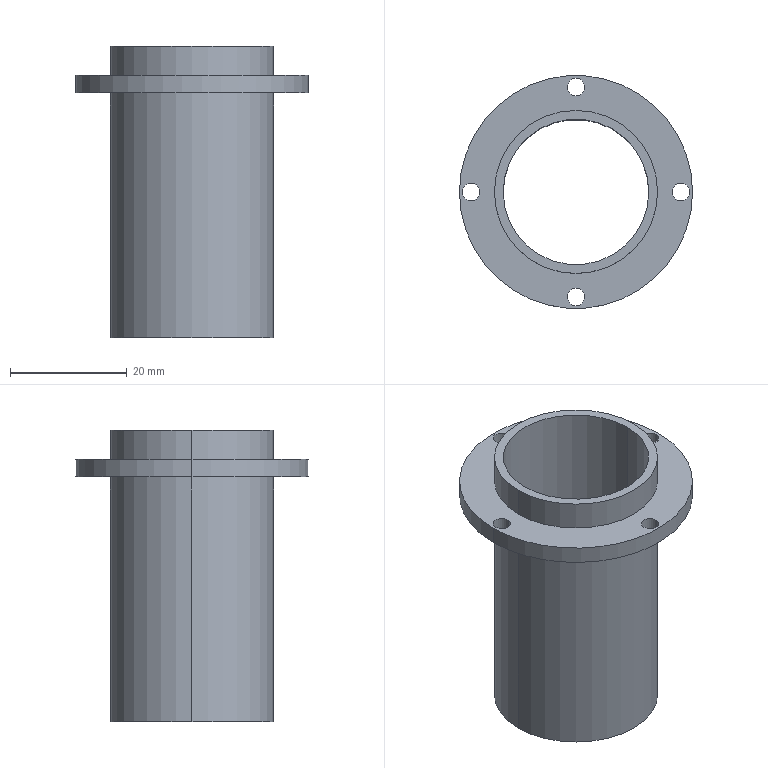Part | SolidWorks | features Extrusion 1, ICE 1 | 1 solid | 20 faces | box 40 x 40 x 50 mm | volume 8082 mm3 | cylinder 16 | plane 4 | commonest cylinder face diameters 3 x8 28 x4 25 x2 40 x2
STEP:
#1=CARTESIAN_POINT('',(-19.5,0.,17.));
#2=VERTEX_POINT('',#1);
#3=CARTESIAN_POINT('',(-16.5,0.,17.));
#4=VERTEX_POINT('',#3);
#5=CARTESIAN_POINT('',(-18.,0.,17.));
#6=DIRECTION('',(0.,0.,1.));
#7=DIRECTION('',(1.,0.,0.));
#8=AXIS2_PLACEMENT_3D('',#5,#6,#7);
#9=CIRCLE('',#8,1.5);
#10=EDGE_CURVE('',#2,#4,#9,.T.);
#11=ORIENTED_EDGE('',*,*,#10,.F.);
#12=CARTESIAN_POINT('',(-19.5,0.,20.));
#13=VERTEX_POINT('',#12);
#14=CARTESIAN_POINT('',(-19.5,0.,17.));
#15=DIRECTION('',(0.,0.,1.));
#16=VECTOR('',#15,1000.);
#17=LINE('',#14,#16);
#18=EDGE_CURVE('',#2,#13,#17,.T.);
#19=ORIENTED_EDGE('',*,*,#18,.T.);
#20=CARTESIAN_POINT('',(-16.5,0.,20.));
#21=VERTEX_POINT('',#20);
#22=CARTESIAN_POINT('',(-18.,0.,20.));
#23=DIRECTION('',(0.,0.,1.));
#24=DIRECTION('',(1.,0.,0.));
#25=AXIS2_PLACEMENT_3D('',#22,#23,#24);
#26=CIRCLE('',#25,1.5);
#27=EDGE_CURVE('',#13,#21,#26,.T.);
#28=ORIENTED_EDGE('',*,*,#27,.T.);
#29=CARTESIAN_POINT('',(-16.5,0.,17.));
#30=DIRECTION('',(0.,0.,1.));
#31=VECTOR('',#30,1000.);
#32=LINE('',#29,#31);
#33=EDGE_CURVE('',#4,#21,#32,.T.);
#34=ORIENTED_EDGE('',*,*,#33,.F.);
#35=EDGE_LOOP('',(#11,#19,#28,#34));
#36=FACE_OUTER_BOUND('',#35,.T.);
#37=CARTESIAN_POINT('',(-18.,0.,17.));
#38=DIRECTION('',(0.,0.,1.));
#39=DIRECTION('',(1.,0.,0.));
#40=AXIS2_PLACEMENT_3D('',#37,#38,#39);
#41=CYLINDRICAL_SURFACE('',#40,1.5);
#42=ADVANCED_FACE('',(#36),#41,.F.);
#43=CARTESIAN_POINT('',(-1.5,-18.,17.));
#44=VERTEX_POINT('',#43);
#45=CARTESIAN_POINT('',(1.5,-18.,17.));
#46=VERTEX_POINT('',#45);
#47=CARTESIAN_POINT('',(0.,-18.,17.));
#48=DIRECTION('',(0.,0.,1.));
#49=DIRECTION('',(1.,0.,0.));
#50=AXIS2_PLACEMENT_3D('',#47,#48,#49);
#51=CIRCLE('',#50,1.5);
#52=EDGE_CURVE('',#44,#46,#51,.T.);
#53=ORIENTED_EDGE('',*,*,#52,.F.);
#54=CARTESIAN_POINT('',(-1.5,-18.,20.));
#55=VERTEX_POINT('',#54);
#56=CARTESIAN_POINT('',(-1.5,-18.,17.));
#57=DIRECTION('',(0.,0.,1.));
#58=VECTOR('',#57,1000.);
#59=LINE('',#56,#58);
#60=EDGE_CURVE('',#44,#55,#59,.T.);
#61=ORIENTED_EDGE('',*,*,#60,.T.);
#62=CARTESIAN_POINT('',(1.5,-18.,20.));
#63=VERTEX_POINT('',#62);
#64=CARTESIAN_POINT('',(0.,-18.,20.));
#65=DIRECTION('',(0.,0.,1.));
#66=DIRECTION('',(1.,0.,0.));
#67=AXIS2_PLACEMENT_3D('',#64,#65,#66);
#68=CIRCLE('',#67,1.5);
#69=EDGE_CURVE('',#55,#63,#68,.T.);
#70=ORIENTED_EDGE('',*,*,#69,.T.);
#71=CARTESIAN_POINT('',(1.5,-18.,17.));
#72=DIRECTION('',(0.,0.,1.));
#73=VECTOR('',#72,1000.);
#74=LINE('',#71,#73);
#75=EDGE_CURVE('',#46,#63,#74,.T.);
#76=ORIENTED_EDGE('',*,*,#75,.F.);
#77=EDGE_LOOP('',(#53,#61,#70,#76));
#78=FACE_OUTER_BOUND('',#77,.T.);
#79=CARTESIAN_POINT('',(0.,-18.,17.));
#80=DIRECTION('',(0.,0.,1.));
#81=DIRECTION('',(1.,0.,0.));
#82=AXIS2_PLACEMENT_3D('',#79,#80,#81);
#83=CYLINDRICAL_SURFACE('',#82,1.5);
#84=ADVANCED_FACE('',(#78),#83,.F.);
#85=CARTESIAN_POINT('',(16.5,0.,17.));
#86=VERTEX_POINT('',#85);
#87=CARTESIAN_POINT('',(19.5,0.,17.));
#88=VERTEX_POINT('',#87);
#89=CARTESIAN_POINT('',(18.,0.,17.));
#90=DIRECTION('',(0.,0.,1.));
#91=DIRECTION('',(1.,0.,0.));
#92=AXIS2_PLACEMENT_3D('',#89,#90,#91);
#93=CIRCLE('',#92,1.5);
#94=EDGE_CURVE('',#86,#88,#93,.T.);
#95=ORIENTED_EDGE('',*,*,#94,.F.);
#96=CARTESIAN_POINT('',(16.5,0.,20.));
#97=VERTEX_POINT('',#96);
#98=CARTESIAN_POINT('',(16.5,0.,17.));
#99=DIRECTION('',(0.,0.,1.));
#100=VECTOR('',#99,1000.);
#101=LINE('',#98,#100);
#102=EDGE_CURVE('',#86,#97,#101,.T.);
#103=ORIENTED_EDGE('',*,*,#102,.T.);
#104=CARTESIAN_POINT('',(19.5,0.,20.));
#105=VERTEX_POINT('',#104);
#106=CARTESIAN_POINT('',(18.,0.,20.));
#107=DIRECTION('',(0.,0.,1.));
#108=DIRECTION('',(1.,0.,0.));
#109=AXIS2_PLACEMENT_3D('',#106,#107,#108);
#110=CIRCLE('',#109,1.5);
#111=EDGE_CURVE('',#97,#105,#110,.T.);
#112=ORIENTED_EDGE('',*,*,#111,.T.);
#113=CARTESIAN_POINT('',(19.5,0.,17.));
#114=DIRECTION('',(0.,0.,1.));
#115=VECTOR('',#114,1000.);
#116=LINE('',#113,#115);
#117=EDGE_CURVE('',#88,#105,#116,.T.);
#118=ORIENTED_EDGE('',*,*,#117,.F.);
#119=EDGE_LOOP('',(#95,#103,#112,#118));
#120=FACE_OUTER_BOUND('',#119,.T.);
#121=CARTESIAN_POINT('',(18.,0.,17.));
#122=DIRECTION('',(0.,0.,1.));
#123=DIRECTION('',(1.,0.,0.));
#124=AXIS2_PLACEMENT_3D('',#121,#122,#123);
#125=CYLINDRICAL_SURFACE('',#124,1.5);
#126=ADVANCED_FACE('',(#120),#125,.F.);
#127=CARTESIAN_POINT('',(-1.5,18.,17.));
#128=VERTEX_POINT('',#127);
#129=CARTESIAN_POINT('',(1.5,18.,17.));
#130=VERTEX_POINT('',#129);
#131=CARTESIAN_POINT('',(0.,18.,17.));
#132=DIRECTION('',(0.,0.,1.));
#133=DIRECTION('',(1.,0.,0.));
#134=AXIS2_PLACEMENT_3D('',#131,#132,#133);
#135=CIRCLE('',#134,1.5);
#136=EDGE_CURVE('',#128,#130,#135,.T.);
#137=ORIENTED_EDGE('',*,*,#136,.F.);
#138=CARTESIAN_POINT('',(-1.5,18.,20.));
#139=VERTEX_POINT('',#138);
#140=CARTESIAN_POINT('',(-1.5,18.,17.));
#141=DIRECTION('',(0.,0.,1.));
#142=VECTOR('',#141,1000.);
#143=LINE('',#140,#142);
#144=EDGE_CURVE('',#128,#139,#143,.T.);
#145=ORIENTED_EDGE('',*,*,#144,.T.);
#146=CARTESIAN_POINT('',(1.5,18.,20.));
#147=VERTEX_POINT('',#146);
#148=CARTESIAN_POINT('',(0.,18.,20.));
#149=DIRECTION('',(0.,0.,1.));
#150=DIRECTION('',(1.,0.,0.));
#151=AXIS2_PLACEMENT_3D('',#148,#149,#150);
#152=CIRCLE('',#151,1.5);
#153=EDGE_CURVE('',#139,#147,#152,.T.);
#154=ORIENTED_EDGE('',*,*,#153,.T.);
#155=CARTESIAN_POINT('',(1.5,18.,17.));
#156=DIRECTION('',(0.,0.,1.));
#157=VECTOR('',#156,1000.);
#158=LINE('',#155,#157);
#159=EDGE_CURVE('',#130,#147,#158,.T.);
#160=ORIENTED_EDGE('',*,*,#159,.F.);
#161=EDGE_LOOP('',(#137,#145,#154,#160));
#162=FACE_OUTER_BOUND('',#161,.T.);
#163=CARTESIAN_POINT('',(0.,18.,17.));
#164=DIRECTION('',(0.,0.,1.));
#165=DIRECTION('',(1.,0.,0.));
#166=AXIS2_PLACEMENT_3D('',#163,#164,#165);
#167=CYLINDRICAL_SURFACE('',#166,1.5);
#168=ADVANCED_FACE('',(#162),#167,.F.);
#169=CARTESIAN_POINT('',(20.,0.,17.));
#170=VERTEX_POINT('',#169);
#171=CARTESIAN_POINT('',(-20.,0.,17.));
#172=VERTEX_POINT('',#171);
#173=CARTESIAN_POINT('',(0.,0.,17.));
#174=DIRECTION('',(0.,0.,1.));
#175=DIRECTION('',(1.,0.,0.));
#176=AXIS2_PLACEMENT_3D('',#173,#174,#175);
#177=CIRCLE('',#176,20.);
#178=EDGE_CURVE('',#170,#172,#177,.T.);
#179=ORIENTED_EDGE('',*,*,#178,.T.);
#180=CARTESIAN_POINT('',(-20.,0.,20.));
#181=VERTEX_POINT('',#180);
#182=CARTESIAN_POINT('',(-20.,0.,17.));
#183=DIRECTION('',(0.,0.,1.));
#184=VECTOR('',#183,1000.);
#185=LINE('',#182,#184);
#186=EDGE_CURVE('',#172,#181,#185,.T.);
#187=ORIENTED_EDGE('',*,*,#186,.T.);
#188=CARTESIAN_POINT('',(20.,0.,20.));
#189=VERTEX_POINT('',#188);
#190=CARTESIAN_POINT('',(0.,0.,20.));
#191=DIRECTION('',(0.,0.,1.));
#192=DIRECTION('',(1.,0.,0.));
#193=AXIS2_PLACEMENT_3D('',#190,#191,#192);
#194=CIRCLE('',#193,20.);
#195=EDGE_CURVE('',#189,#181,#194,.T.);
#196=ORIENTED_EDGE('',*,*,#195,.F.);
#197=CARTESIAN_POINT('',(20.,0.,17.));
#198=DIRECTION('',(0.,0.,1.));
#199=VECTOR('',#198,1000.);
#200=LINE('',#197,#199);
#201=EDGE_CURVE('',#170,#189,#200,.T.);
#202=ORIENTED_EDGE('',*,*,#201,.F.);
#203=EDGE_LOOP('',(#179,#187,#196,#202));
#204=FACE_OUTER_BOUND('',#203,.T.);
#205=CARTESIAN_POINT('',(0.,0.,17.));
#206=DIRECTION('',(0.,0.,1.));
#207=DIRECTION('',(1.,0.,0.));
#208=AXIS2_PLACEMENT_3D('',#205,#206,#207);
#209=CYLINDRICAL_SURFACE('',#208,20.);
#210=ADVANCED_FACE('',(#204),#209,.T.);
#211=CARTESIAN_POINT('',(-12.5,0.,25.));
#212=VERTEX_POINT('',#211);
#213=CARTESIAN_POINT('',(12.5,0.,25.));
#214=VERTEX_POINT('',#213);
#215=CARTESIAN_POINT('',(0.,0.,25.));
#216=DIRECTION('',(0.,0.,1.));
#217=DIRECTION('',(1.,0.,0.));
#218=AXIS2_PLACEMENT_3D('',#215,#216,#217);
#219=CIRCLE('',#218,12.5);
#220=EDGE_CURVE('',#212,#214,#219,.T.);
#221=ORIENTED_EDGE('',*,*,#220,.T.);
#222=CARTESIAN_POINT('',(12.5,0.,-25.));
#223=VERTEX_POINT('',#222);
#224=CARTESIAN_POINT('',(12.5,0.,25.));
#225=DIRECTION('',(0.,0.,-1.));
#226=VECTOR('',#225,1000.);
#227=LINE('',#224,#226);
#228=EDGE_CURVE('',#214,#223,#227,.T.);
#229=ORIENTED_EDGE('',*,*,#228,.T.);
#230=CARTESIAN_POINT('',(-12.5,0.,-25.));
#231=VERTEX_POINT('',#230);
#232=CARTESIAN_POINT('',(0.,0.,-25.));
#233=DIRECTION('',(0.,0.,1.));
#234=DIRECTION('',(1.,0.,0.));
#235=AXIS2_PLACEMENT_3D('',#232,#233,#234);
#236=CIRCLE('',#235,12.5);
#237=EDGE_CURVE('',#231,#223,#236,.T.);
#238=ORIENTED_EDGE('',*,*,#237,.F.);
#239=CARTESIAN_POINT('',(-12.5,0.,25.));
#240=DIRECTION('',(0.,0.,-1.));
#241=VECTOR('',#240,1000.);
#242=LINE('',#239,#241);
#243=EDGE_CURVE('',#212,#231,#242,.T.);
#244=ORIENTED_EDGE('',*,*,#243,.F.);
#245=EDGE_LOOP('',(#221,#229,#238,#244));
#246=FACE_OUTER_BOUND('',#245,.T.);
#247=CARTESIAN_POINT('',(0.,0.,25.));
#248=DIRECTION('',(0.,0.,-1.));
#249=DIRECTION('',(-1.,0.,0.));
#250=AXIS2_PLACEMENT_3D('',#247,#248,#249);
#251=CYLINDRICAL_SURFACE('',#250,12.5);
#252=ADVANCED_FACE('',(#246),#251,.F.);
#253=CARTESIAN_POINT('',(14.,0.,25.));
#254=VERTEX_POINT('',#253);
#255=CARTESIAN_POINT('',(-14.,0.,25.));
#256=VERTEX_POINT('',#255);
#257=CARTESIAN_POINT('',(0.,0.,25.));
#258=DIRECTION('',(0.,0.,1.));
#259=DIRECTION('',(1.,0.,0.));
#260=AXIS2_PLACEMENT_3D('',#257,#258,#259);
#261=CIRCLE('',#260,14.);
#262=EDGE_CURVE('',#254,#256,#261,.T.);
#263=ORIENTED_EDGE('',*,*,#262,.F.);
#264=CARTESIAN_POINT('',(14.,0.,20.));
#265=VERTEX_POINT('',#264);
#266=CARTESIAN_POINT('',(14.,0.,25.));
#267=DIRECTION('',(0.,0.,-1.));
#268=VECTOR('',#267,1000.);
#269=LINE('',#266,#268);
#270=EDGE_CURVE('',#254,#265,#269,.T.);
#271=ORIENTED_EDGE('',*,*,#270,.T.);
#272=CARTESIAN_POINT('',(-14.,0.,20.));
#273=VERTEX_POINT('',#272);
#274=CARTESIAN_POINT('',(0.,0.,20.));
#275=DIRECTION('',(0.,0.,1.));
#276=DIRECTION('',(1.,0.,0.));
#277=AXIS2_PLACEMENT_3D('',#274,#275,#276);
#278=CIRCLE('',#277,14.);
#279=EDGE_CURVE('',#265,#273,#278,.T.);
#280=ORIENTED_EDGE('',*,*,#279,.T.);
#281=CARTESIAN_POINT('',(-14.,0.,25.));
#282=DIRECTION('',(0.,0.,-1.));
#283=VECTOR('',#282,1000.);
#284=LINE('',#281,#283);
#285=EDGE_CURVE('',#256,#273,#284,.T.);
#286=ORIENTED_EDGE('',*,*,#285,.F.);
#287=EDGE_LOOP('',(#263,#271,#280,#286));
#288=FACE_OUTER_BOUND('',#287,.T.);
#289=CARTESIAN_POINT('',(0.,0.,25.));
#290=DIRECTION('',(0.,0.,-1.));
#291=DIRECTION('',(-1.,0.,0.));
#292=AXIS2_PLACEMENT_3D('',#289,#290,#291);
#293=CYLINDRICAL_SURFACE('',#292,14.);
#294=ADVANCED_FACE('',(#288),#293,.T.);
#295=CARTESIAN_POINT('',(14.,0.,17.));
#296=VERTEX_POINT('',#295);
#297=CARTESIAN_POINT('',(-14.,0.,17.));
#298=VERTEX_POINT('',#297);
#299=CARTESIAN_POINT('',(0.,0.,17.));
#300=DIRECTION('',(0.,0.,1.));
#301=DIRECTION('',(1.,0.,0.));
#302=AXIS2_PLACEMENT_3D('',#299,#300,#301);
#303=CIRCLE('',#302,14.);
#304=EDGE_CURVE('',#296,#298,#303,.T.);
#305=ORIENTED_EDGE('',*,*,#304,.F.);
#306=CARTESIAN_POINT('',(14.,0.,-25.));
#307=VERTEX_POINT('',#306);
#308=CARTESIAN_POINT('',(14.,0.,25.));
#309=DIRECTION('',(0.,0.,-1.));
#310=VECTOR('',#309,1000.);
#311=LINE('',#308,#310);
#312=EDGE_CURVE('',#296,#307,#311,.T.);
#313=ORIENTED_EDGE('',*,*,#312,.T.);
#314=CARTESIAN_POINT('',(-14.,0.,-25.));
#315=VERTEX_POINT('',#314);
#316=CARTESIAN_POINT('',(0.,0.,-25.));
#317=DIRECTION('',(0.,0.,1.));
#318=DIRECTION('',(1.,0.,0.));
#319=AXIS2_PLACEMENT_3D('',#316,#317,#318);
#320=CIRCLE('',#319,14.);
#321=EDGE_CURVE('',#307,#315,#320,.T.);
#322=ORIENTED_EDGE('',*,*,#321,.T.);
#323=CARTESIAN_POINT('',(-14.,0.,25.));
#324=DIRECTION('',(0.,0.,-1.));
#325=VECTOR('',#324,1000.);
#326=LINE('',#323,#325);
#327=EDGE_CURVE('',#298,#315,#326,.T.);
#328=ORIENTED_EDGE('',*,*,#327,.F.);
#329=EDGE_LOOP('',(#305,#313,#322,#328));
#330=FACE_OUTER_BOUND('',#329,.T.);
#331=CARTESIAN_POINT('',(0.,0.,25.));
#332=DIRECTION('',(0.,0.,-1.));
#333=DIRECTION('',(-1.,0.,0.));
#334=AXIS2_PLACEMENT_3D('',#331,#332,#333);
#335=CYLINDRICAL_SURFACE('',#334,14.);
#336=ADVANCED_FACE('',(#330),#335,.T.);
#337=ORIENTED_EDGE('',*,*,#312,.F.);
#338=CARTESIAN_POINT('',(0.,0.,17.));
#339=DIRECTION('',(0.,0.,1.));
#340=DIRECTION('',(1.,0.,0.));
#341=AXIS2_PLACEMENT_3D('',#338,#339,#340);
#342=CIRCLE('',#341,14.);
#343=EDGE_CURVE('',#298,#296,#342,.T.);
#344=ORIENTED_EDGE('',*,*,#343,.F.);
#345=ORIENTED_EDGE('',*,*,#327,.T.);
#346=CARTESIAN_POINT('',(0.,0.,-25.));
#347=DIRECTION('',(0.,0.,1.));
#348=DIRECTION('',(1.,0.,0.));
#349=AXIS2_PLACEMENT_3D('',#346,#347,#348);
#350=CIRCLE('',#349,14.);
#351=EDGE_CURVE('',#315,#307,#350,.T.);
#352=ORIENTED_EDGE('',*,*,#351,.T.);
#353=EDGE_LOOP('',(#337,#344,#345,#352));
#354=FACE_OUTER_BOUND('',#353,.T.);
#355=CARTESIAN_POINT('',(0.,0.,25.));
#356=DIRECTION('',(0.,0.,-1.));
#357=DIRECTION('',(-1.,0.,0.));
#358=AXIS2_PLACEMENT_3D('',#355,#356,#357);
#359=CYLINDRICAL_SURFACE('',#358,14.);
#360=ADVANCED_FACE('',(#354),#359,.T.);
#361=CARTESIAN_POINT('',(0.,0.,25.));
#362=DIRECTION('',(0.,0.,1.));
#363=DIRECTION('',(1.,0.,0.));
#364=AXIS2_PLACEMENT_3D('',#361,#362,#363);
#365=CIRCLE('',#364,14.);
#366=EDGE_CURVE('',#256,#254,#365,.T.);
#367=ORIENTED_EDGE('',*,*,#366,.T.);
#368=ORIENTED_EDGE('',*,*,#262,.T.);
#369=EDGE_LOOP('',(#367,#368));
#370=FACE_OUTER_BOUND('',#369,.T.);
#371=ORIENTED_EDGE('',*,*,#220,.F.);
#372=CARTESIAN_POINT('',(0.,0.,25.));
#373=DIRECTION('',(0.,0.,1.));
#374=DIRECTION('',(1.,0.,0.));
#375=AXIS2_PLACEMENT_3D('',#372,#373,#374);
#376=CIRCLE('',#375,12.5);
#377=EDGE_CURVE('',#214,#212,#376,.T.);
#378=ORIENTED_EDGE('',*,*,#377,.F.);
#379=EDGE_LOOP('',(#371,#378));
#380=FACE_BOUND('',#379,.T.);
#381=CARTESIAN_POINT('',(0.,0.,25.));
#382=DIRECTION('',(0.,0.,1.));
#383=DIRECTION('',(1.,0.,0.));
#384=AXIS2_PLACEMENT_3D('',#381,#382,#383);
#385=PLANE('',#384);
#386=ADVANCED_FACE('',(#370,#380),#385,.T.);
#387=ORIENTED_EDGE('',*,*,#351,.F.);
#388=ORIENTED_EDGE('',*,*,#321,.F.);
#389=EDGE_LOOP('',(#387,#388));
#390=FACE_OUTER_BOUND('',#389,.T.);
#391=ORIENTED_EDGE('',*,*,#237,.T.);
#392=CARTESIAN_POINT('',(0.,0.,-25.));
#393=DIRECTION('',(0.,0.,1.));
#394=DIRECTION('',(1.,0.,0.));
#395=AXIS2_PLACEMENT_3D('',#392,#393,#394);
#396=CIRCLE('',#395,12.5);
#397=EDGE_CURVE('',#223,#231,#396,.T.);
#398=ORIENTED_EDGE('',*,*,#397,.T.);
#399=EDGE_LOOP('',(#391,#398));
#400=FACE_BOUND('',#399,.T.);
#401=CARTESIAN_POINT('',(0.,0.,-25.));
#402=DIRECTION('',(0.,0.,1.));
#403=DIRECTION('',(1.,0.,0.));
#404=AXIS2_PLACEMENT_3D('',#401,#402,#403);
#405=PLANE('',#404);
#406=ADVANCED_FACE('',(#390,#400),#405,.F.);
#407=ORIENTED_EDGE('',*,*,#270,.F.);
#408=ORIENTED_EDGE('',*,*,#366,.F.);
#409=ORIENTED_EDGE('',*,*,#285,.T.);
#410=CARTESIAN_POINT('',(0.,0.,20.));
#411=DIRECTION('',(0.,0.,1.));
#412=DIRECTION('',(1.,0.,0.));
#413=AXIS2_PLACEMENT_3D('',#410,#411,#412);
#414=CIRCLE('',#413,14.);
#415=EDGE_CURVE('',#273,#265,#414,.T.);
#416=ORIENTED_EDGE('',*,*,#415,.T.);
#417=EDGE_LOOP('',(#407,#408,#409,#416));
#418=FACE_OUTER_BOUND('',#417,.T.);
#419=CARTESIAN_POINT('',(0.,0.,25.));
#420=DIRECTION('',(0.,0.,-1.));
#421=DIRECTION('',(-1.,0.,0.));
#422=AXIS2_PLACEMENT_3D('',#419,#420,#421);
#423=CYLINDRICAL_SURFACE('',#422,14.);
#424=ADVANCED_FACE('',(#418),#423,.T.);
#425=ORIENTED_EDGE('',*,*,#228,.F.);
#426=ORIENTED_EDGE('',*,*,#377,.T.);
#427=ORIENTED_EDGE('',*,*,#243,.T.);
#428=ORIENTED_EDGE('',*,*,#397,.F.);
#429=EDGE_LOOP('',(#425,#426,#427,#428));
#430=FACE_OUTER_BOUND('',#429,.T.);
#431=CARTESIAN_POINT('',(0.,0.,25.));
#432=DIRECTION('',(0.,0.,-1.));
#433=DIRECTION('',(-1.,0.,0.));
#434=AXIS2_PLACEMENT_3D('',#431,#432,#433);
#435=CYLINDRICAL_SURFACE('',#434,12.5);
#436=ADVANCED_FACE('',(#430),#435,.F.);
#437=ORIENTED_EDGE('',*,*,#178,.F.);
#438=CARTESIAN_POINT('',(0.,0.,17.));
#439=DIRECTION('',(0.,0.,1.));
#440=DIRECTION('',(1.,0.,0.));
#441=AXIS2_PLACEMENT_3D('',#438,#439,#440);
#442=CIRCLE('',#441,20.);
#443=EDGE_CURVE('',#172,#170,#442,.T.);
#444=ORIENTED_EDGE('',*,*,#443,.F.);
#445=EDGE_LOOP('',(#437,#444));
#446=FACE_OUTER_BOUND('',#445,.T.);
#447=CARTESIAN_POINT('',(0.,18.,17.));
#448=DIRECTION('',(0.,0.,1.));
#449=DIRECTION('',(1.,0.,0.));
#450=AXIS2_PLACEMENT_3D('',#447,#448,#449);
#451=CIRCLE('',#450,1.5);
#452=EDGE_CURVE('',#130,#128,#451,.T.);
#453=ORIENTED_EDGE('',*,*,#452,.T.);
#454=ORIENTED_EDGE('',*,*,#136,.T.);
#455=EDGE_LOOP('',(#453,#454));
#456=FACE_BOUND('',#455,.T.);
#457=CARTESIAN_POINT('',(18.,0.,17.));
#458=DIRECTION('',(0.,0.,1.));
#459=DIRECTION('',(1.,0.,0.));
#460=AXIS2_PLACEMENT_3D('',#457,#458,#459);
#461=CIRCLE('',#460,1.5);
#462=EDGE_CURVE('',#88,#86,#461,.T.);
#463=ORIENTED_EDGE('',*,*,#462,.T.);
#464=ORIENTED_EDGE('',*,*,#94,.T.);
#465=EDGE_LOOP('',(#463,#464));
#466=FACE_BOUND('',#465,.T.);
#467=CARTESIAN_POINT('',(0.,-18.,17.));
#468=DIRECTION('',(0.,0.,1.));
#469=DIRECTION('',(1.,0.,0.));
#470=AXIS2_PLACEMENT_3D('',#467,#468,#469);
#471=CIRCLE('',#470,1.5);
#472=EDGE_CURVE('',#46,#44,#471,.T.);
#473=ORIENTED_EDGE('',*,*,#472,.T.);
#474=ORIENTED_EDGE('',*,*,#52,.T.);
#475=EDGE_LOOP('',(#473,#474));
#476=FACE_BOUND('',#475,.T.);
#477=CARTESIAN_POINT('',(-18.,0.,17.));
#478=DIRECTION('',(0.,0.,1.));
#479=DIRECTION('',(1.,0.,0.));
#480=AXIS2_PLACEMENT_3D('',#477,#478,#479);
#481=CIRCLE('',#480,1.5);
#482=EDGE_CURVE('',#4,#2,#481,.T.);
#483=ORIENTED_EDGE('',*,*,#482,.T.);
#484=ORIENTED_EDGE('',*,*,#10,.T.);
#485=EDGE_LOOP('',(#483,#484));
#486=FACE_BOUND('',#485,.T.);
#487=ORIENTED_EDGE('',*,*,#343,.T.);
#488=ORIENTED_EDGE('',*,*,#304,.T.);
#489=EDGE_LOOP('',(#487,#488));
#490=FACE_BOUND('',#489,.T.);
#491=CARTESIAN_POINT('',(0.,0.,17.));
#492=DIRECTION('',(0.,0.,1.));
#493=DIRECTION('',(1.,0.,0.));
#494=AXIS2_PLACEMENT_3D('',#491,#492,#493);
#495=PLANE('',#494);
#496=ADVANCED_FACE('',(#446,#456,#466,#476,#486,#490),#495,.F.);
#497=ORIENTED_EDGE('',*,*,#195,.T.);
#498=CARTESIAN_POINT('',(0.,0.,20.));
#499=DIRECTION('',(0.,0.,1.));
#500=DIRECTION('',(1.,0.,0.));
#501=AXIS2_PLACEMENT_3D('',#498,#499,#500);
#502=CIRCLE('',#501,20.);
#503=EDGE_CURVE('',#181,#189,#502,.T.);
#504=ORIENTED_EDGE('',*,*,#503,.T.);
#505=EDGE_LOOP('',(#497,#504));
#506=FACE_OUTER_BOUND('',#505,.T.);
#507=CARTESIAN_POINT('',(0.,18.,20.));
#508=DIRECTION('',(0.,0.,1.));
#509=DIRECTION('',(1.,0.,0.));
#510=AXIS2_PLACEMENT_3D('',#507,#508,#509);
#511=CIRCLE('',#510,1.5);
#512=EDGE_CURVE('',#147,#139,#511,.T.);
#513=ORIENTED_EDGE('',*,*,#512,.F.);
#514=ORIENTED_EDGE('',*,*,#153,.F.);
#515=EDGE_LOOP('',(#513,#514));
#516=FACE_BOUND('',#515,.T.);
#517=CARTESIAN_POINT('',(18.,0.,20.));
#518=DIRECTION('',(0.,0.,1.));
#519=DIRECTION('',(1.,0.,0.));
#520=AXIS2_PLACEMENT_3D('',#517,#518,#519);
#521=CIRCLE('',#520,1.5);
#522=EDGE_CURVE('',#105,#97,#521,.T.);
#523=ORIENTED_EDGE('',*,*,#522,.F.);
#524=ORIENTED_EDGE('',*,*,#111,.F.);
#525=EDGE_LOOP('',(#523,#524));
#526=FACE_BOUND('',#525,.T.);
#527=CARTESIAN_POINT('',(0.,-18.,20.));
#528=DIRECTION('',(0.,0.,1.));
#529=DIRECTION('',(1.,0.,0.));
#530=AXIS2_PLACEMENT_3D('',#527,#528,#529);
#531=CIRCLE('',#530,1.5);
#532=EDGE_CURVE('',#63,#55,#531,.T.);
#533=ORIENTED_EDGE('',*,*,#532,.F.);
#534=ORIENTED_EDGE('',*,*,#69,.F.);
#535=EDGE_LOOP('',(#533,#534));
#536=FACE_BOUND('',#535,.T.);
#537=CARTESIAN_POINT('',(-18.,0.,20.));
#538=DIRECTION('',(0.,0.,1.));
#539=DIRECTION('',(1.,0.,0.));
#540=AXIS2_PLACEMENT_3D('',#537,#538,#539);
#541=CIRCLE('',#540,1.5);
#542=EDGE_CURVE('',#21,#13,#541,.T.);
#543=ORIENTED_EDGE('',*,*,#542,.F.);
#544=ORIENTED_EDGE('',*,*,#27,.F.);
#545=EDGE_LOOP('',(#543,#544));
#546=FACE_BOUND('',#545,.T.);
#547=ORIENTED_EDGE('',*,*,#415,.F.);
#548=ORIENTED_EDGE('',*,*,#279,.F.);
#549=EDGE_LOOP('',(#547,#548));
#550=FACE_BOUND('',#549,.T.);
#551=CARTESIAN_POINT('',(0.,0.,20.));
#552=DIRECTION('',(0.,0.,1.));
#553=DIRECTION('',(1.,0.,0.));
#554=AXIS2_PLACEMENT_3D('',#551,#552,#553);
#555=PLANE('',#554);
#556=ADVANCED_FACE('',(#506,#516,#526,#536,#546,#550),#555,.T.);
#557=ORIENTED_EDGE('',*,*,#186,.F.);
#558=ORIENTED_EDGE('',*,*,#443,.T.);
#559=ORIENTED_EDGE('',*,*,#201,.T.);
#560=ORIENTED_EDGE('',*,*,#503,.F.);
#561=EDGE_LOOP('',(#557,#558,#559,#560));
#562=FACE_OUTER_BOUND('',#561,.T.);
#563=CARTESIAN_POINT('',(0.,0.,17.));
#564=DIRECTION('',(0.,0.,1.));
#565=DIRECTION('',(1.,0.,0.));
#566=AXIS2_PLACEMENT_3D('',#563,#564,#565);
#567=CYLINDRICAL_SURFACE('',#566,20.);
#568=ADVANCED_FACE('',(#562),#567,.T.);
#569=ORIENTED_EDGE('',*,*,#144,.F.);
#570=ORIENTED_EDGE('',*,*,#452,.F.);
#571=ORIENTED_EDGE('',*,*,#159,.T.);
#572=ORIENTED_EDGE('',*,*,#512,.T.);
#573=EDGE_LOOP('',(#569,#570,#571,#572));
#574=FACE_OUTER_BOUND('',#573,.T.);
#575=CARTESIAN_POINT('',(0.,18.,17.));
#576=DIRECTION('',(0.,0.,1.));
#577=DIRECTION('',(1.,0.,0.));
#578=AXIS2_PLACEMENT_3D('',#575,#576,#577);
#579=CYLINDRICAL_SURFACE('',#578,1.5);
#580=ADVANCED_FACE('',(#574),#579,.F.);
#581=ORIENTED_EDGE('',*,*,#102,.F.);
#582=ORIENTED_EDGE('',*,*,#462,.F.);
#583=ORIENTED_EDGE('',*,*,#117,.T.);
#584=ORIENTED_EDGE('',*,*,#522,.T.);
#585=EDGE_LOOP('',(#581,#582,#583,#584));
#586=FACE_OUTER_BOUND('',#585,.T.);
#587=CARTESIAN_POINT('',(18.,0.,17.));
#588=DIRECTION('',(0.,0.,1.));
#589=DIRECTION('',(1.,0.,0.));
#590=AXIS2_PLACEMENT_3D('',#587,#588,#589);
#591=CYLINDRICAL_SURFACE('',#590,1.5);
#592=ADVANCED_FACE('',(#586),#591,.F.);
#593=ORIENTED_EDGE('',*,*,#60,.F.);
#594=ORIENTED_EDGE('',*,*,#472,.F.);
#595=ORIENTED_EDGE('',*,*,#75,.T.);
#596=ORIENTED_EDGE('',*,*,#532,.T.);
#597=EDGE_LOOP('',(#593,#594,#595,#596));
#598=FACE_OUTER_BOUND('',#597,.T.);
#599=CARTESIAN_POINT('',(0.,-18.,17.));
#600=DIRECTION('',(0.,0.,1.));
#601=DIRECTION('',(1.,0.,0.));
#602=AXIS2_PLACEMENT_3D('',#599,#600,#601);
#603=CYLINDRICAL_SURFACE('',#602,1.5);
#604=ADVANCED_FACE('',(#598),#603,.F.);
#605=ORIENTED_EDGE('',*,*,#18,.F.);
#606=ORIENTED_EDGE('',*,*,#482,.F.);
#607=ORIENTED_EDGE('',*,*,#33,.T.);
#608=ORIENTED_EDGE('',*,*,#542,.T.);
#609=EDGE_LOOP('',(#605,#606,#607,#608));
#610=FACE_OUTER_BOUND('',#609,.T.);
#611=CARTESIAN_POINT('',(-18.,0.,17.));
#612=DIRECTION('',(0.,0.,1.));
#613=DIRECTION('',(1.,0.,0.));
#614=AXIS2_PLACEMENT_3D('',#611,#612,#613);
#615=CYLINDRICAL_SURFACE('',#614,1.5);
#616=ADVANCED_FACE('',(#610),#615,.F.);
#617=CLOSED_SHELL('',(#42,#84,#126,#168,#210,#252,#294,#336,#360,#386,#406,#424,#436,#496,#556,#568,#580,#592,#604,#616));
#618=MANIFOLD_SOLID_BREP('',#617);
#619=CARTESIAN_POINT('',(0.,0.,0.));
#620=DIRECTION('',(0.,0.,1.));
#621=DIRECTION('',(1.,0.,0.));
#622=AXIS2_PLACEMENT_3D('',#619,#620,#621);
#623=(LENGTH_UNIT()NAMED_UNIT(*)SI_UNIT(.MILLI.,.METRE.));
#624=UNCERTAINTY_MEASURE_WITH_UNIT(LENGTH_MEASURE(0.00001),#623,'','');
#625=(NAMED_UNIT(*)PLANE_ANGLE_UNIT()SI_UNIT($,.RADIAN.));
#626=(NAMED_UNIT(*)SI_UNIT($,.STERADIAN.)SOLID_ANGLE_UNIT());
#627=(GEOMETRIC_REPRESENTATION_CONTEXT(3)GLOBAL_UNCERTAINTY_ASSIGNED_CONTEXT((#624))GLOBAL_UNIT_ASSIGNED_CONTEXT((#623,#625,#626))REPRESENTATION_CONTEXT('',''));
#628=ADVANCED_BREP_SHAPE_REPRESENTATION('',(#618,#622),#627);